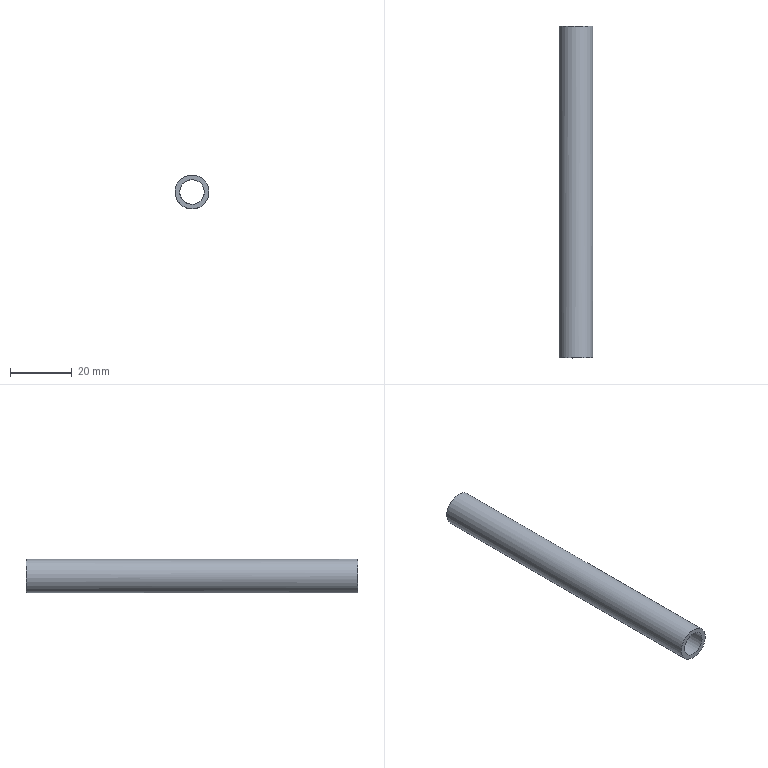Part | NX | features solid 2 | 1 solid | 4 faces | box 11 x 107.645 x 11 mm | volume 4818 mm3 | cylinder 2 | plane 1 | spline 1 | commonest cylinder face diameters 8 x1 11 x1
STEP:
#1=CARTESIAN_POINT('',(16.,-330.,351.));
#2=VERTEX_POINT('',#1);
#3=CARTESIAN_POINT('',(16.,-330.,347.));
#4=DIRECTION('',(0.,1.,0.));
#5=DIRECTION('',(0.,0.,1.));
#6=AXIS2_PLACEMENT_3D('',#3,#4,#5);
#7=CIRCLE('',#6,4.);
#8=EDGE_CURVE('',#2,#2,#7,.T.);
#9=ORIENTED_EDGE('',*,*,#8,.T.);
#10=EDGE_LOOP('',(#9));
#11=FACE_BOUND('',#10,.T.);
#12=CARTESIAN_POINT('',(15.96,-437.644,343.));
#13=VERTEX_POINT('',#12);
#14=CARTESIAN_POINT('',(19.106,-437.643,343.837));
#15=CARTESIAN_POINT('',(15.955,-437.644,342.566));
#16=CARTESIAN_POINT('',(12.834,-437.645,343.899));
#17=CARTESIAN_POINT('',(11.568,-437.645,347.041));
#18=CARTESIAN_POINT('',(12.895,-437.645,350.164));
#19=CARTESIAN_POINT('',(16.044,-437.644,351.432));
#20=CARTESIAN_POINT('',(19.162,-437.643,350.106));
#21=CARTESIAN_POINT('',(20.433,-437.642,346.96));
#22=CARTESIAN_POINT('',(19.106,-437.643,343.837));
#23=CARTESIAN_POINT('',(15.955,-437.644,342.566));
#24=CARTESIAN_POINT('',(12.834,-437.645,343.899));
#25=B_SPLINE_CURVE_WITH_KNOTS('',3,(#14,#15,#16,#17,#18,#19,#20,#21,#22,#23,#24),.UNSPECIFIED.,.T.,.F.,(1,1,1,1,1,1,1,1,1,1,1,1,1,1,1),(-0.009378,-0.006252,-0.003126,0.,0.003126,0.006252,0.009378,0.0125,0.01563,0.01876,0.02188,0.02501,0.02813,0.03126,0.03439),.UNSPECIFIED.);
#26=EDGE_CURVE('',#13,#13,#25,.T.);
#27=ORIENTED_EDGE('',*,*,#26,.F.);
#28=EDGE_LOOP('',(#27));
#29=FACE_BOUND('',#28,.T.);
#30=CARTESIAN_POINT('',(16.,-330.,347.));
#31=DIRECTION('',(0.,-1.,0.));
#32=DIRECTION('',(0.,0.,-1.));
#33=AXIS2_PLACEMENT_3D('',#30,#31,#32);
#34=CYLINDRICAL_SURFACE('',#33,4.);
#35=ADVANCED_FACE('',(#11,#29),#34,.F.);
#36=CARTESIAN_POINT('',(16.,-330.,352.5));
#37=VERTEX_POINT('',#36);
#38=CARTESIAN_POINT('',(16.,-330.,347.));
#39=DIRECTION('',(0.,1.,0.));
#40=DIRECTION('',(0.,0.,1.));
#41=AXIS2_PLACEMENT_3D('',#38,#39,#40);
#42=CIRCLE('',#41,5.5);
#43=EDGE_CURVE('',#37,#37,#42,.T.);
#44=ORIENTED_EDGE('',*,*,#43,.F.);
#45=EDGE_LOOP('',(#44));
#46=FACE_BOUND('',#45,.T.);
#47=CARTESIAN_POINT('',(15.96,-437.644,341.5));
#48=VERTEX_POINT('',#47);
#49=CARTESIAN_POINT('',(20.283,-437.642,342.662));
#50=CARTESIAN_POINT('',(15.954,-437.644,340.904));
#51=CARTESIAN_POINT('',(11.658,-437.645,342.724));
#52=CARTESIAN_POINT('',(9.906,-437.645,347.04));
#53=CARTESIAN_POINT('',(11.719,-437.645,351.339));
#54=CARTESIAN_POINT('',(16.044,-437.644,353.094));
#55=CARTESIAN_POINT('',(20.336,-437.642,351.283));
#56=CARTESIAN_POINT('',(22.095,-437.64,346.962));
#57=CARTESIAN_POINT('',(20.283,-437.642,342.662));
#58=CARTESIAN_POINT('',(15.954,-437.644,340.904));
#59=CARTESIAN_POINT('',(11.658,-437.645,342.724));
#60=B_SPLINE_CURVE_WITH_KNOTS('',3,(#49,#50,#51,#52,#53,#54,#55,#56,#57,#58,#59),.UNSPECIFIED.,.T.,.F.,(1,1,1,1,1,1,1,1,1,1,1,1,1,1,1),(-0.0129,-0.008597,-0.004298,0.,0.004298,0.008597,0.0129,0.01719,0.02149,0.02579,0.03009,0.03439,0.03869,0.04298,0.04728),.UNSPECIFIED.);
#61=EDGE_CURVE('',#48,#48,#60,.T.);
#62=ORIENTED_EDGE('',*,*,#61,.T.);
#63=EDGE_LOOP('',(#62));
#64=FACE_BOUND('',#63,.T.);
#65=CARTESIAN_POINT('',(16.,-330.,347.));
#66=DIRECTION('',(0.,-1.,0.));
#67=DIRECTION('',(0.,0.,-1.));
#68=AXIS2_PLACEMENT_3D('',#65,#66,#67);
#69=CYLINDRICAL_SURFACE('',#68,5.5);
#70=ADVANCED_FACE('',(#46,#64),#69,.T.);
#71=ORIENTED_EDGE('',*,*,#8,.F.);
#72=EDGE_LOOP('',(#71));
#73=FACE_BOUND('',#72,.T.);
#74=ORIENTED_EDGE('',*,*,#43,.T.);
#75=EDGE_LOOP('',(#74));
#76=FACE_BOUND('',#75,.T.);
#77=CARTESIAN_POINT('',(16.,-330.,347.));
#78=DIRECTION('',(0.,1.,0.));
#79=DIRECTION('',(0.,0.,1.));
#80=AXIS2_PLACEMENT_3D('',#77,#78,#79);
#81=PLANE('',#80);
#82=ADVANCED_FACE('',(#73,#76),#81,.T.);
#83=ORIENTED_EDGE('',*,*,#26,.T.);
#84=EDGE_LOOP('',(#83));
#85=FACE_BOUND('',#84,.T.);
#86=ORIENTED_EDGE('',*,*,#61,.F.);
#87=EDGE_LOOP('',(#86));
#88=FACE_BOUND('',#87,.T.);
#89=CARTESIAN_POINT('',(10.4,-437.645,352.6));
#90=CARTESIAN_POINT('',(10.4,-437.645,341.431));
#91=CARTESIAN_POINT('',(14.121,-437.645,352.6));
#92=CARTESIAN_POINT('',(14.121,-437.645,341.431));
#93=CARTESIAN_POINT('',(17.847,-437.644,352.6));
#94=CARTESIAN_POINT('',(17.847,-437.644,341.431));
#95=CARTESIAN_POINT('',(21.577,-437.641,352.6));
#96=CARTESIAN_POINT('',(21.577,-437.641,341.431));
#97=B_SPLINE_SURFACE_WITH_KNOTS('',3,1,((#89,#90),(#91,#92),(#93,#94),(#95,#96)),.SURF_OF_LINEAR_EXTRUSION.,.F.,.F.,.F.,(4,4),(2,2),(0.5039,0.5062),(0.,1.),.PIECEWISE_BEZIER_KNOTS.);
#98=ADVANCED_FACE('',(#85,#88),#97,.F.);
#99=CLOSED_SHELL('',(#35,#70,#82,#98));
#100=MANIFOLD_SOLID_BREP('',#99);
#101=(LENGTH_UNIT()NAMED_UNIT(*)SI_UNIT(.MILLI.,.METRE.));
#102=UNCERTAINTY_MEASURE_WITH_UNIT(LENGTH_MEASURE(0.0508),#101,'','');
#103=(NAMED_UNIT(*)PLANE_ANGLE_UNIT()SI_UNIT($,.RADIAN.));
#104=(NAMED_UNIT(*)SI_UNIT($,.STERADIAN.)SOLID_ANGLE_UNIT());
#105=(GEOMETRIC_REPRESENTATION_CONTEXT(3)GLOBAL_UNCERTAINTY_ASSIGNED_CONTEXT((#102))GLOBAL_UNIT_ASSIGNED_CONTEXT((#101,#103,#104))REPRESENTATION_CONTEXT('',''));
#106=ADVANCED_BREP_SHAPE_REPRESENTATION('',(#100),#105);